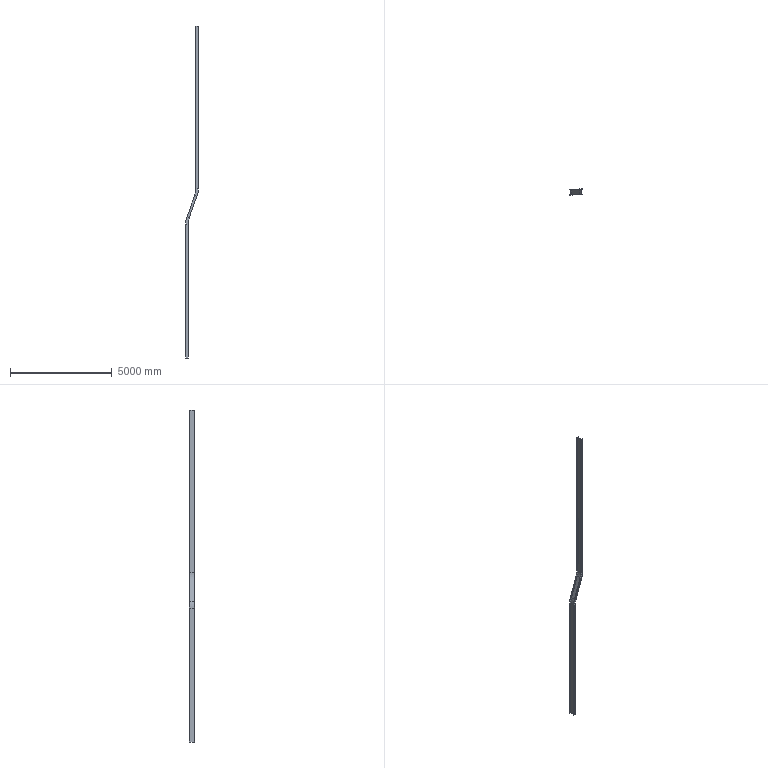Part | SolidWorks | features Sweep 1 | 1 solid | 102 faces | box 622 x 280 x 16285 mm | volume 87987824 mm3 | plane 42 | cylinder 36 | torus 16 | cone 8 | commonest cylinder face diameters 10.6 x12 21 x12 1758 x4 2002 x4 1872 x2 1888 x2